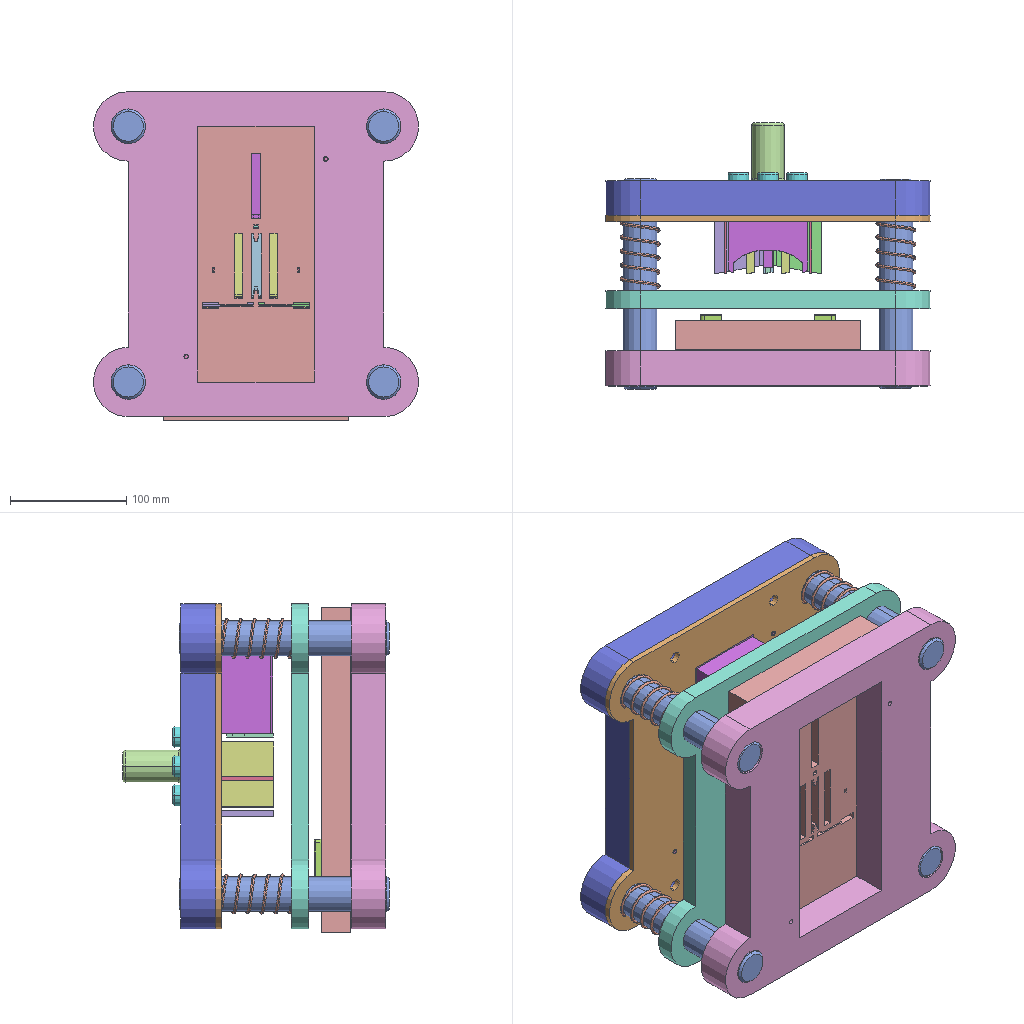Assembly | SolidWorks | 18 different items | 33 placed | box 279 x 229 x 283 mm
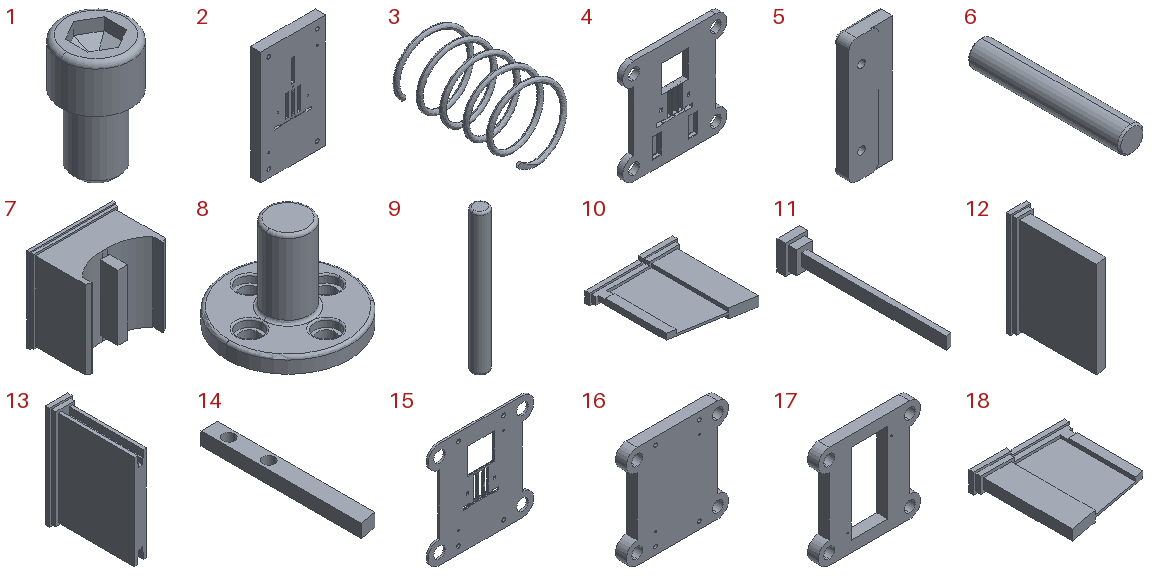Parts list (item | quantity | size | volume | features):
1 | x4 | 18 x 18 x 30 mm | 4675 mm3 | features Chamfer 2, Fillet 2, ICE 2, Extrusion 1, RefAxis 1
2 | x1 | 160 x 25 x 280 mm | 1024971 mm3 | features Cut 5, ICE 2, Extrusion 1, HoleWzd 1
3 | x4 | 34.5 x 60 x 34.5 mm | 2448 mm3 | features Helix 1, ICE 1, Sweep 1
4 | x1 | 280 x 15 x 280 mm | 817644 mm3 | features Cut 2, Extrusion 1, Fillet 1, MirrorPattern 1
5 | x2 | 18 x 6 x 50 mm | 5021 mm3 | features Fillet 4, ICE 3, Extrusion 1
6 | x4 | 30 x 178 x 30 mm | 125461 mm3 | features Chamfer 1, Revolution 1
7 | x1 | 73.144 x 49.228 x 71.78 mm | 167014 mm3 | features ICE 4, Extrusion 1
8 | x1 | 80 x 80 x 60 mm | 74517 mm3 | features Fillet 4, ICE 3, Extrusion 1
9 | x4 | 4 x 4 x 35 mm | 438.55 mm3 | features Extrusion 1, Fillet 1
10 | x1 | 48.36 x 50 x 10.06 mm | 6665 mm3 | features ICE 4, Extrusion 1
11 | x2 | 7 x 50 x 9 mm | 546.722 mm3 | features ICE 3, Extrusion 1
12 | x2 | 11.5 x 50 x 61 mm | 18724 mm3 | features ICE 3, Extrusion 1
13 | x1 | 13.06 x 50 x 60.56 mm | 21649 mm3 | features ICE 3, Extrusion 1
14 | x1 | 4.18 x 40 x 3.28 mm | 496.993 mm3 | features ICE 2, Extrusion 1
15 | x1 | 280 x 5 x 280 mm | 281508 mm3 | features ICE 6, Extrusion 1
16 | x1 | 280 x 30 x 280 mm | 1868516 mm3 | features ICE 4, Extrusion 1, Fillet 1, HoleWzd 1, MirrorPattern 1
17 | x1 | 280 x 30 x 280 mm | 1265786 mm3 | features ICE 2, Extrusion 1, HoleWzd 1, MirrorPattern 1
18 | x1 | 48.36 x 50 x 10.06 mm | 6665 mm3 | features ICE 4, Extrusion 1
Mates (type | each side: item.copy, entity, surface, feature):
Concentric | 2.1 edge | 5.1 edge
Coincident | 2.1 face plane Boss-Extrude1 | 5.1 face plane Boss-Extrude1
Concentric | 6.1 edge | 17.1 edge
Coincident | 6.1 face plane Revolve1 | 17.1 face plane Boss-Extrude1
Concentric | 6.1 face cylinder Revolve1 | 4.1 edge
Concentric | 6.1 face cylinder Revolve1 | 15.1 edge
Coincident | 15.1 face plane Cut-Extrude1 | 18.1 face plane Boss-Extrude3 | 3 times
Coincident | 15.1 face plane Cut-Extrude1 | 10.1 face plane Boss-Extrude3 | 3 times
Coincident | 15.1 face plane Cut-Extrude1 | 11.1 face plane Boss-Extrude3 | 3 times
Coincident | 15.1 face plane Cut-Extrude1 | 11.2 face plane Boss-Extrude3 | 3 times
Coincident | 15.1 face plane Cut-Extrude1 | 13.1 face plane Boss-Extrude3 | 3 times
Coincident | 15.1 edge | 12.1 face plane Boss-Extrude3
Coincident | 15.1 face plane Cut-Extrude1 | 12.1 face plane Boss-Extrude3 | 2 times
Coincident | 15.1 face plane Cut-Extrude1 | 12.2 face plane Boss-Extrude3 | 3 times
Coincident | 7.1 face plane Boss-Extrude1 | 14.1 face plane Boss-Extrude1
Concentric | 7.1 edge | 14.1 edge
Coincident | 15.1 face plane Cut-Extrude1 | 7.1 face plane Boss-Extrude5 | 3 times
Concentric | 6.2 face cylinder Revolve1 | 17.1 edge
Concentric | 6.3 face cylinder Revolve1 | 17.1 edge
Concentric | 6.4 face cylinder Revolve1 | 17.1 edge
Concentric | 2.1 edge | 17.1 face cylinder Cut-Extrude1
Concentric | 15.1 face cylinder Boss-Extrude1 | 16.1 edge
Coincident | 15.1 face plane Boss-Extrude1 | 16.1 face plane Boss-Extrude1
Coincident | 16.1 face plane Cut-Extrude4 | 8.1 face plane Boss-Extrude1
Concentric | 16.1 edge | 8.1 edge
Concentric | 6.1 face cylinder Revolve1 | 3.1 select_type:24
Coincident | 4.1 face plane Boss-Extrude1 | 3.1 select_type:24
Coincident | 4.1 face plane Boss-Extrude1 | 3.2 select_type:24
Coincident | 4.1 face plane Boss-Extrude1 | 3.3 select_type:24
Concentric | 6.2 face cylinder Revolve1 | 3.3 select_type:24
Concentric | 6.3 face cylinder Revolve1 | 3.2 select_type:24
Coincident | 4.1 face plane Boss-Extrude1 | 3.4 select_type:24
Concentric | 6.4 face cylinder Revolve1 | 3.4 select_type:24
Coincident | 6.2 face plane Revolve1 | 17.1 face plane Boss-Extrude1
DistanceDim | 15.1 face plane Boss-Extrude1 | 4.1 face plane Boss-Extrude1
Concentric | 16.1 edge | 9.1 face cylinder Boss-Extrude1
Concentric | 16.1 edge | 9.1 edge
Coincident | 16.1 face plane Boss-Extrude1 | 9.1 face plane Boss-Extrude1
Concentric | 16.1 face cylinder Cut-Extrude1 | 9.2 face cylinder Boss-Extrude1
Coincident | 16.1 face plane Boss-Extrude1 | 9.2 face plane Boss-Extrude1
Concentric | 17.1 face cylinder Cut-Extrude2 | 9.3 face cylinder Boss-Extrude1
Coincident | 2.1 face plane Boss-Extrude1 | 9.3 face plane Boss-Extrude1
Concentric | 17.1 face cylinder Cut-Extrude2 | 9.4 face cylinder Boss-Extrude1
Coincident | 2.1 face plane Boss-Extrude1 | 9.4 face plane Boss-Extrude1
Coincident | 8.1 face plane Cut-Extrude1 | 1.1 plane
Concentric | 16.1 face cylinder Cut-Extrude7 | 1.1 axis
Coincident | 8.1 face plane Cut-Extrude1 | 1.2 plane
Concentric | 16.1 face cylinder Cut-Extrude7 | 1.2 axis
Coincident | 8.1 face plane Cut-Extrude1 | 1.3 plane
Concentric | 8.1 face cylinder Cut-Extrude2 | 1.3 axis
Coincident | 8.1 face plane Cut-Extrude1 | 1.4 plane
Concentric | 16.1 face cylinder Cut-Extrude7 | 1.4 axis